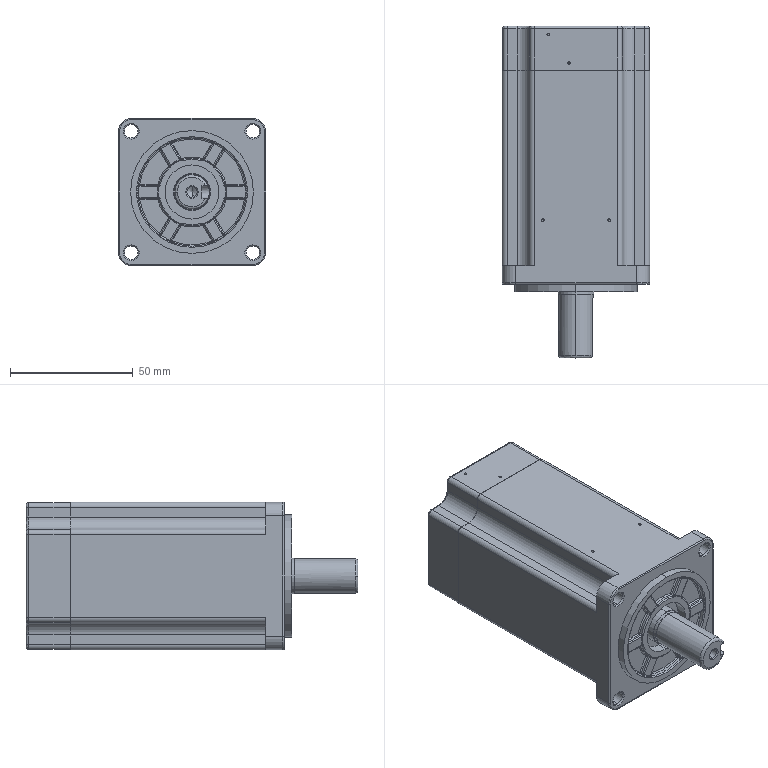Part | SolidWorks | features BaseBody 1 | 1 solid | 445 faces | box 60 x 135 x 60 mm | volume 337667 mm3 | spline 226 | cylinder 139 | plane 68 | cone 12 | commonest cylinder face diameters 1 x56 2 x12 3.8 x8 4 x8 5.5 x8 27.6 x7